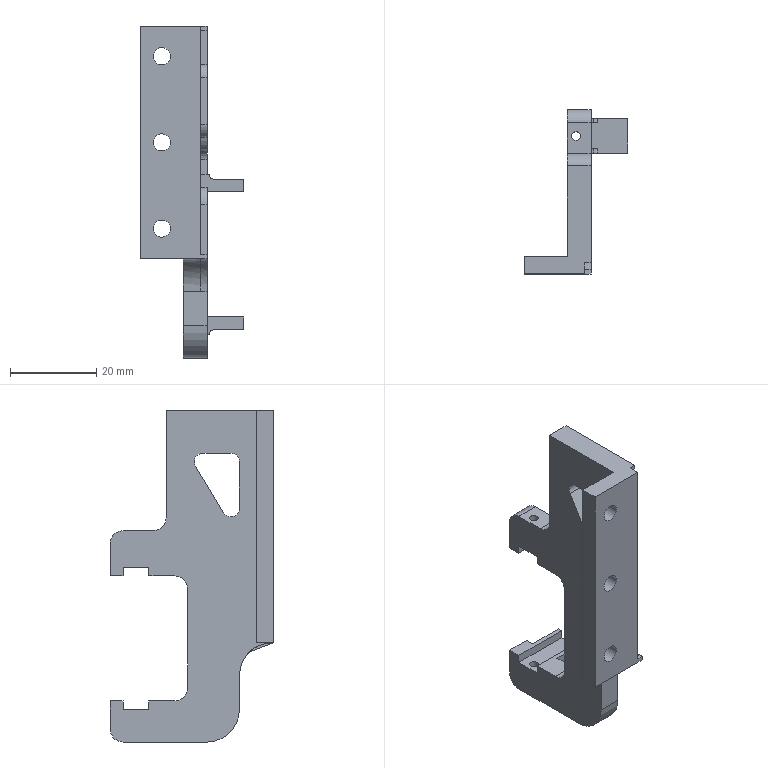Part | STEP file | 1-09.1 | 1 solid | 95 faces | box 24 x 38 x 77 mm | volume 9451 mm3 | plane 65 | cylinder 30 | commonest cylinder face diameters 4 x8 6 x8 2 x6 8 x3 15 x2 13 x1